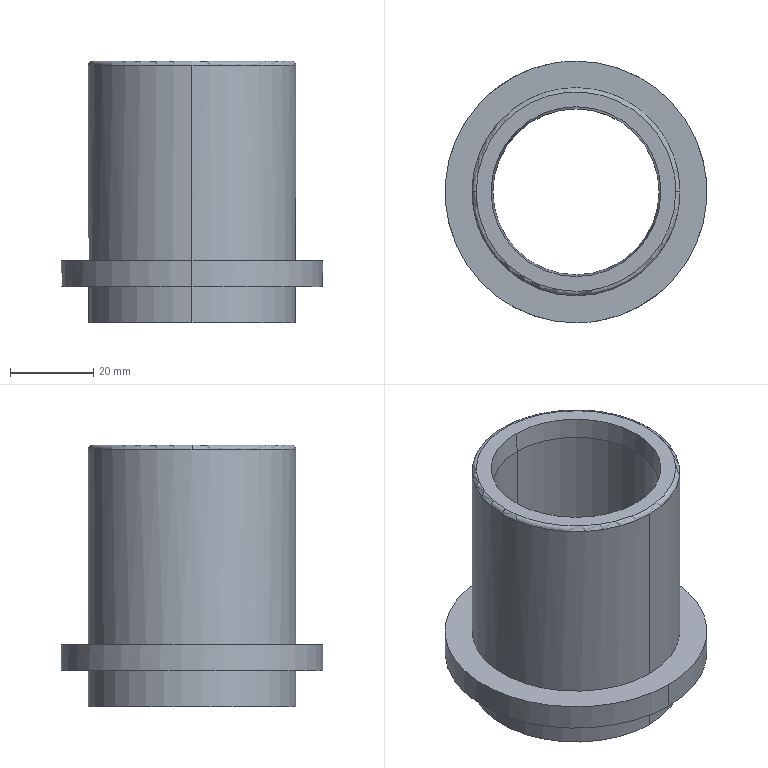Part | CATIA | 1 solid | 18 faces | box 63 x 63 x 63 mm | volume 51378 mm3 | cylinder 8 | plane 4 | torus 4 | cone 2 | commonest cylinder face diameters 50 x4 40 x2 63 x2
STEP:
#1=CARTESIAN_POINT('',(0.,-20.437,48.));
#2=VERTEX_POINT('',#1);
#3=CARTESIAN_POINT('',(0.,-20.,43.));
#4=VERTEX_POINT('',#3);
#5=CARTESIAN_POINT('',(0.,-43587.981,498027.299));
#6=DIRECTION('',(0.,-0.08716,0.9962));
#7=VECTOR('',#6,1.);
#8=LINE('',#5,#7);
#9=EDGE_CURVE('',#2,#4,#8,.F.);
#10=ORIENTED_EDGE('',*,*,#9,.F.);
#11=CARTESIAN_POINT('',(0.,20.437,48.));
#12=VERTEX_POINT('',#11);
#13=CARTESIAN_POINT('',(0.,0.,48.));
#14=DIRECTION('',(0.,0.,1.));
#15=AXIS2_PLACEMENT_3D('',#13,#14,$);
#16=CIRCLE('',#15,20.437);
#17=EDGE_CURVE('',#12,#2,#16,.F.);
#18=ORIENTED_EDGE('',*,*,#17,.F.);
#19=CARTESIAN_POINT('',(0.,20.,43.));
#20=VERTEX_POINT('',#19);
#21=CARTESIAN_POINT('',(0.,43587.981,498027.299));
#22=DIRECTION('',(0.,0.08716,0.9962));
#23=VECTOR('',#22,1.);
#24=LINE('',#21,#23);
#25=EDGE_CURVE('',#20,#12,#24,.T.);
#26=ORIENTED_EDGE('',*,*,#25,.F.);
#27=CARTESIAN_POINT('',(0.,0.,43.));
#28=DIRECTION('',(0.,0.,1.));
#29=AXIS2_PLACEMENT_3D('',#27,#28,$);
#30=CIRCLE('',#29,20.);
#31=EDGE_CURVE('',#20,#4,#30,.F.);
#32=ORIENTED_EDGE('',*,*,#31,.T.);
#33=EDGE_LOOP('',(#10,#18,#26,#32));
#34=FACE_OUTER_BOUND('',#33,.T.);
#35=CARTESIAN_POINT('',(0.,0.,45.5));
#36=DIRECTION('',(0.,0.,1.));
#37=DIRECTION('',(0.,-1.,0.));
#38=AXIS2_PLACEMENT_3D('',#35,#36,#37);
#39=CONICAL_SURFACE('',#38,20.219,0.08727);
#40=ADVANCED_FACE('',(#34),#39,.F.);
#41=ORIENTED_EDGE('',*,*,#9,.T.);
#42=CARTESIAN_POINT('',(0.,0.,43.));
#43=DIRECTION('',(0.,0.,1.));
#44=AXIS2_PLACEMENT_3D('',#42,#43,$);
#45=CIRCLE('',#44,20.);
#46=EDGE_CURVE('',#4,#20,#45,.F.);
#47=ORIENTED_EDGE('',*,*,#46,.T.);
#48=ORIENTED_EDGE('',*,*,#25,.T.);
#49=CARTESIAN_POINT('',(0.,0.,48.));
#50=DIRECTION('',(0.,0.,1.));
#51=AXIS2_PLACEMENT_3D('',#49,#50,$);
#52=CIRCLE('',#51,20.437);
#53=EDGE_CURVE('',#2,#12,#52,.F.);
#54=ORIENTED_EDGE('',*,*,#53,.F.);
#55=EDGE_LOOP('',(#41,#47,#48,#54));
#56=FACE_OUTER_BOUND('',#55,.T.);
#57=CARTESIAN_POINT('',(0.,0.,45.5));
#58=DIRECTION('',(0.,0.,1.));
#59=DIRECTION('',(0.,1.,0.));
#60=AXIS2_PLACEMENT_3D('',#57,#58,#59);
#61=CONICAL_SURFACE('',#60,20.219,0.08727);
#62=ADVANCED_FACE('',(#56),#61,.F.);
#63=CARTESIAN_POINT('',(0.,-24.,48.));
#64=VERTEX_POINT('',#63);
#65=CARTESIAN_POINT('',(-24.,-0.000000001,48.));
#66=VERTEX_POINT('',#65);
#67=CARTESIAN_POINT('',(0.,-24.,48.));
#68=CARTESIAN_POINT('',(-2.4,-24.,48.));
#69=CARTESIAN_POINT('',(-4.8,-23.7,48.));
#70=CARTESIAN_POINT('',(-7.15,-23.1,48.));
#71=CARTESIAN_POINT('',(-11.65,-21.325,48.));
#72=CARTESIAN_POINT('',(-15.575,-18.498,48.));
#73=CARTESIAN_POINT('',(-17.349,-16.844,48.));
#74=CARTESIAN_POINT('',(-20.448,-13.129,48.));
#75=CARTESIAN_POINT('',(-22.536,-8.766,48.));
#76=CARTESIAN_POINT('',(-23.301,-6.464,48.));
#77=CARTESIAN_POINT('',(-23.836,-3.756,48.));
#78=CARTESIAN_POINT('',(-23.982,-1.02,48.));
#79=CARTESIAN_POINT('',(-23.994,-0.6796,48.));
#80=CARTESIAN_POINT('',(-24.,-0.3398,48.));
#81=CARTESIAN_POINT('',(-24.,-0.000000001,48.));
#82=B_SPLINE_CURVE_WITH_KNOTS('',5,(#67,#68,#69,#70,#71,#72,#73,#74,#75,#76,#77,#78,#79,#80,#81),.UNSPECIFIED.,.F.,.U.,(6,3,3,3,6),(0.,17.012,34.025,51.037,53.446),.UNSPECIFIED.);
#83=EDGE_CURVE('',#64,#66,#82,.T.);
#84=ORIENTED_EDGE('',*,*,#83,.F.);
#85=CARTESIAN_POINT('',(24.,-0.000000001,48.));
#86=VERTEX_POINT('',#85);
#87=CARTESIAN_POINT('',(24.,-0.000000001,48.));
#88=CARTESIAN_POINT('',(24.,-2.4,48.));
#89=CARTESIAN_POINT('',(23.7,-4.8,48.));
#90=CARTESIAN_POINT('',(23.1,-7.15,48.));
#91=CARTESIAN_POINT('',(21.325,-11.65,48.));
#92=CARTESIAN_POINT('',(18.498,-15.575,48.));
#93=CARTESIAN_POINT('',(16.844,-17.349,48.));
#94=CARTESIAN_POINT('',(13.129,-20.448,48.));
#95=CARTESIAN_POINT('',(8.766,-22.536,48.));
#96=CARTESIAN_POINT('',(6.464,-23.301,48.));
#97=CARTESIAN_POINT('',(3.756,-23.836,48.));
#98=CARTESIAN_POINT('',(1.02,-23.982,48.));
#99=CARTESIAN_POINT('',(0.6796,-23.994,48.));
#100=CARTESIAN_POINT('',(0.3398,-24.,48.));
#101=CARTESIAN_POINT('',(0.,-24.,48.));
#102=B_SPLINE_CURVE_WITH_KNOTS('',5,(#87,#88,#89,#90,#91,#92,#93,#94,#95,#96,#97,#98,#99,#100,#101),.UNSPECIFIED.,.F.,.U.,(6,3,3,3,6),(0.,17.012,34.025,51.037,53.446),.UNSPECIFIED.);
#103=EDGE_CURVE('',#86,#64,#102,.T.);
#104=ORIENTED_EDGE('',*,*,#103,.F.);
#105=CARTESIAN_POINT('',(-24.,-0.000000001,48.));
#106=CARTESIAN_POINT('',(-24.,2.4,48.));
#107=CARTESIAN_POINT('',(-23.7,4.8,48.));
#108=CARTESIAN_POINT('',(-23.1,7.15,48.));
#109=CARTESIAN_POINT('',(-21.325,11.65,48.));
#110=CARTESIAN_POINT('',(-18.498,15.575,48.));
#111=CARTESIAN_POINT('',(-16.844,17.349,48.));
#112=CARTESIAN_POINT('',(-13.129,20.448,48.));
#113=CARTESIAN_POINT('',(-8.766,22.536,48.));
#114=CARTESIAN_POINT('',(-6.464,23.301,48.));
#115=CARTESIAN_POINT('',(-1.719,24.239,48.));
#116=CARTESIAN_POINT('',(3.111,23.98,48.));
#117=CARTESIAN_POINT('',(5.498,23.548,48.));
#118=CARTESIAN_POINT('',(10.112,22.096,48.));
#119=CARTESIAN_POINT('',(14.227,19.553,48.));
#120=CARTESIAN_POINT('',(16.114,18.029,48.));
#121=CARTESIAN_POINT('',(19.468,14.543,48.));
#122=CARTESIAN_POINT('',(21.86,10.339,48.));
#123=CARTESIAN_POINT('',(22.785,8.097,48.));
#124=CARTESIAN_POINT('',(23.601,5.103,48.));
#125=CARTESIAN_POINT('',(23.928,2.039,48.));
#126=CARTESIAN_POINT('',(23.976,1.359,48.));
#127=CARTESIAN_POINT('',(24.,0.6793,48.));
#128=CARTESIAN_POINT('',(24.,-0.000000001,48.));
#129=B_SPLINE_CURVE_WITH_KNOTS('',5,(#105,#106,#107,#108,#109,#110,#111,#112,#113,#114,#115,#116,#117,#118,#119,#120,#121,#122,#123,#124,#125,#126,#127,#128),.UNSPECIFIED.,.F.,.U.,(6,3,3,3,3,3,3,6),(0.,17.013,34.025,51.038,68.051,85.063,102.076,106.892),.UNSPECIFIED.);
#130=EDGE_CURVE('',#66,#86,#129,.T.);
#131=ORIENTED_EDGE('',*,*,#130,.F.);
#132=EDGE_LOOP('',(#84,#104,#131));
#133=FACE_OUTER_BOUND('',#132,.T.);
#134=ORIENTED_EDGE('',*,*,#53,.T.);
#135=ORIENTED_EDGE('',*,*,#17,.T.);
#136=EDGE_LOOP('',(#134,#135));
#137=FACE_BOUND('',#136,.T.);
#138=CARTESIAN_POINT('',(0.,-22.219,48.));
#139=DIRECTION('',(0.,0.,1.));
#140=DIRECTION('',(0.,1.,0.));
#141=AXIS2_PLACEMENT_3D('',#138,#139,#140);
#142=PLANE('',#141);
#143=ADVANCED_FACE('',(#133,#137),#142,.T.);
#144=CARTESIAN_POINT('',(0.,-20.,-12.));
#145=VERTEX_POINT('',#144);
#146=CARTESIAN_POINT('',(0.,-20.,15.5));
#147=DIRECTION('',(0.,0.,1.));
#148=VECTOR('',#147,1.);
#149=LINE('',#146,#148);
#150=EDGE_CURVE('',#4,#145,#149,.F.);
#151=ORIENTED_EDGE('',*,*,#150,.F.);
#152=ORIENTED_EDGE('',*,*,#31,.F.);
#153=CARTESIAN_POINT('',(0.,20.,-12.));
#154=VERTEX_POINT('',#153);
#155=CARTESIAN_POINT('',(0.,20.,15.5));
#156=DIRECTION('',(0.,0.,1.));
#157=VECTOR('',#156,1.);
#158=LINE('',#155,#157);
#159=EDGE_CURVE('',#154,#20,#158,.T.);
#160=ORIENTED_EDGE('',*,*,#159,.F.);
#161=CARTESIAN_POINT('',(20.,0.,-12.));
#162=VERTEX_POINT('',#161);
#163=CARTESIAN_POINT('',(0.,0.,-12.));
#164=DIRECTION('',(0.,0.,1.));
#165=AXIS2_PLACEMENT_3D('',#163,#164,$);
#166=CIRCLE('',#165,20.);
#167=EDGE_CURVE('',#154,#162,#166,.F.);
#168=ORIENTED_EDGE('',*,*,#167,.T.);
#169=CARTESIAN_POINT('',(0.,0.,-12.));
#170=DIRECTION('',(0.,0.,1.));
#171=AXIS2_PLACEMENT_3D('',#169,#170,$);
#172=CIRCLE('',#171,20.);
#173=EDGE_CURVE('',#162,#145,#172,.F.);
#174=ORIENTED_EDGE('',*,*,#173,.T.);
#175=EDGE_LOOP('',(#151,#152,#160,#168,#174));
#176=FACE_OUTER_BOUND('',#175,.T.);
#177=CARTESIAN_POINT('',(0.,0.,15.5));
#178=DIRECTION('',(0.,0.,1.));
#179=DIRECTION('',(0.,-1.,0.));
#180=AXIS2_PLACEMENT_3D('',#177,#178,#179);
#181=CYLINDRICAL_SURFACE('',#180,20.);
#182=ADVANCED_FACE('',(#176),#181,.F.);
#183=ORIENTED_EDGE('',*,*,#150,.T.);
#184=CARTESIAN_POINT('',(-20.,0.,-12.));
#185=VERTEX_POINT('',#184);
#186=CARTESIAN_POINT('',(0.,0.,-12.));
#187=DIRECTION('',(0.,0.,1.));
#188=AXIS2_PLACEMENT_3D('',#186,#187,$);
#189=CIRCLE('',#188,20.);
#190=EDGE_CURVE('',#145,#185,#189,.F.);
#191=ORIENTED_EDGE('',*,*,#190,.T.);
#192=CARTESIAN_POINT('',(0.,0.,-12.));
#193=DIRECTION('',(0.,0.,1.));
#194=AXIS2_PLACEMENT_3D('',#192,#193,$);
#195=CIRCLE('',#194,20.);
#196=EDGE_CURVE('',#185,#154,#195,.F.);
#197=ORIENTED_EDGE('',*,*,#196,.T.);
#198=ORIENTED_EDGE('',*,*,#159,.T.);
#199=ORIENTED_EDGE('',*,*,#46,.F.);
#200=EDGE_LOOP('',(#183,#191,#197,#198,#199));
#201=FACE_OUTER_BOUND('',#200,.T.);
#202=CARTESIAN_POINT('',(0.,0.,15.5));
#203=DIRECTION('',(0.,0.,1.));
#204=DIRECTION('',(0.,1.,0.));
#205=AXIS2_PLACEMENT_3D('',#202,#203,#204);
#206=CYLINDRICAL_SURFACE('',#205,20.);
#207=ADVANCED_FACE('',(#201),#206,.F.);
#208=CARTESIAN_POINT('',(-25.,0.,47.));
#209=VERTEX_POINT('',#208);
#210=CARTESIAN_POINT('',(-24.,0.,47.));
#211=DIRECTION('',(0.,-1.,0.));
#212=AXIS2_PLACEMENT_3D('',#210,#211,$);
#213=CIRCLE('',#212,1.);
#214=EDGE_CURVE('',#66,#209,#213,.T.);
#215=ORIENTED_EDGE('',*,*,#214,.T.);
#216=CARTESIAN_POINT('',(0.,-25.,47.));
#217=VERTEX_POINT('',#216);
#218=CARTESIAN_POINT('',(0.,0.,47.));
#219=DIRECTION('',(0.,0.,-1.));
#220=AXIS2_PLACEMENT_3D('',#218,#219,$);
#221=CIRCLE('',#220,25.);
#222=EDGE_CURVE('',#217,#209,#221,.T.);
#223=ORIENTED_EDGE('',*,*,#222,.F.);
#224=CARTESIAN_POINT('',(25.,0.,47.));
#225=VERTEX_POINT('',#224);
#226=CARTESIAN_POINT('',(0.,0.,47.));
#227=DIRECTION('',(0.,0.,-1.));
#228=AXIS2_PLACEMENT_3D('',#226,#227,$);
#229=CIRCLE('',#228,25.);
#230=EDGE_CURVE('',#225,#217,#229,.T.);
#231=ORIENTED_EDGE('',*,*,#230,.F.);
#232=CARTESIAN_POINT('',(24.,0.,47.));
#233=DIRECTION('',(0.,1.,0.));
#234=AXIS2_PLACEMENT_3D('',#232,#233,$);
#235=CIRCLE('',#234,1.);
#236=EDGE_CURVE('',#225,#86,#235,.F.);
#237=ORIENTED_EDGE('',*,*,#236,.T.);
#238=ORIENTED_EDGE('',*,*,#103,.T.);
#239=ORIENTED_EDGE('',*,*,#83,.T.);
#240=EDGE_LOOP('',(#215,#223,#231,#237,#238,#239));
#241=FACE_OUTER_BOUND('',#240,.T.);
#242=CARTESIAN_POINT('',(0.,0.,47.));
#243=DIRECTION('',(0.,0.,-1.));
#244=DIRECTION('',(1.,0.,0.));
#245=AXIS2_PLACEMENT_3D('',#242,#243,#244);
#246=TOROIDAL_SURFACE('',#245,24.,1.);
#247=ADVANCED_FACE('',(#241),#246,.T.);
#248=ORIENTED_EDGE('',*,*,#214,.F.);
#249=ORIENTED_EDGE('',*,*,#130,.T.);
#250=ORIENTED_EDGE('',*,*,#236,.F.);
#251=CARTESIAN_POINT('',(0.,25.,47.));
#252=VERTEX_POINT('',#251);
#253=CARTESIAN_POINT('',(0.,0.,47.));
#254=DIRECTION('',(0.,0.,-1.));
#255=AXIS2_PLACEMENT_3D('',#253,#254,$);
#256=CIRCLE('',#255,25.);
#257=EDGE_CURVE('',#252,#225,#256,.T.);
#258=ORIENTED_EDGE('',*,*,#257,.F.);
#259=CARTESIAN_POINT('',(0.,0.,47.));
#260=DIRECTION('',(0.,0.,-1.));
#261=AXIS2_PLACEMENT_3D('',#259,#260,$);
#262=CIRCLE('',#261,25.);
#263=EDGE_CURVE('',#209,#252,#262,.T.);
#264=ORIENTED_EDGE('',*,*,#263,.F.);
#265=EDGE_LOOP('',(#248,#249,#250,#258,#264));
#266=FACE_OUTER_BOUND('',#265,.T.);
#267=CARTESIAN_POINT('',(0.,0.,47.));
#268=DIRECTION('',(0.,0.,-1.));
#269=DIRECTION('',(-1.,0.,0.));
#270=AXIS2_PLACEMENT_3D('',#267,#268,#269);
#271=TOROIDAL_SURFACE('',#270,24.,1.);
#272=ADVANCED_FACE('',(#266),#271,.T.);
#273=CARTESIAN_POINT('',(-23.,0.,-15.));
#274=VERTEX_POINT('',#273);
#275=CARTESIAN_POINT('',(-23.,0.,-12.));
#276=DIRECTION('',(0.,-1.,0.));
#277=AXIS2_PLACEMENT_3D('',#275,#276,$);
#278=CIRCLE('',#277,3.);
#279=EDGE_CURVE('',#274,#185,#278,.T.);
#280=ORIENTED_EDGE('',*,*,#279,.F.);
#281=CARTESIAN_POINT('',(23.,0.,-15.));
#282=VERTEX_POINT('',#281);
#283=CARTESIAN_POINT('',(0.,0.,-15.));
#284=DIRECTION('',(0.,0.,-1.));
#285=AXIS2_PLACEMENT_3D('',#283,#284,$);
#286=CIRCLE('',#285,23.);
#287=EDGE_CURVE('',#274,#282,#286,.T.);
#288=ORIENTED_EDGE('',*,*,#287,.T.);
#289=CARTESIAN_POINT('',(23.,0.,-12.));
#290=DIRECTION('',(0.,1.,0.));
#291=AXIS2_PLACEMENT_3D('',#289,#290,$);
#292=CIRCLE('',#291,3.);
#293=EDGE_CURVE('',#162,#282,#292,.F.);
#294=ORIENTED_EDGE('',*,*,#293,.F.);
#295=ORIENTED_EDGE('',*,*,#167,.F.);
#296=ORIENTED_EDGE('',*,*,#196,.F.);
#297=EDGE_LOOP('',(#280,#288,#294,#295,#296));
#298=FACE_OUTER_BOUND('',#297,.T.);
#299=CARTESIAN_POINT('',(0.,0.,-12.));
#300=DIRECTION('',(0.,0.,-1.));
#301=DIRECTION('',(-1.,0.,0.));
#302=AXIS2_PLACEMENT_3D('',#299,#300,#301);
#303=TOROIDAL_SURFACE('',#302,23.,3.);
#304=ADVANCED_FACE('',(#298),#303,.T.);
#305=ORIENTED_EDGE('',*,*,#279,.T.);
#306=ORIENTED_EDGE('',*,*,#190,.F.);
#307=ORIENTED_EDGE('',*,*,#173,.F.);
#308=ORIENTED_EDGE('',*,*,#293,.T.);
#309=CARTESIAN_POINT('',(0.,-23.,-15.));
#310=VERTEX_POINT('',#309);
#311=CARTESIAN_POINT('',(0.,0.,-15.));
#312=DIRECTION('',(0.,0.,-1.));
#313=AXIS2_PLACEMENT_3D('',#311,#312,$);
#314=CIRCLE('',#313,23.);
#315=EDGE_CURVE('',#282,#310,#314,.T.);
#316=ORIENTED_EDGE('',*,*,#315,.T.);
#317=CARTESIAN_POINT('',(0.,0.,-15.));
#318=DIRECTION('',(0.,0.,-1.));
#319=AXIS2_PLACEMENT_3D('',#317,#318,$);
#320=CIRCLE('',#319,23.);
#321=EDGE_CURVE('',#310,#274,#320,.T.);
#322=ORIENTED_EDGE('',*,*,#321,.T.);
#323=EDGE_LOOP('',(#305,#306,#307,#308,#316,#322));
#324=FACE_OUTER_BOUND('',#323,.T.);
#325=CARTESIAN_POINT('',(0.,0.,-12.));
#326=DIRECTION('',(0.,0.,-1.));
#327=DIRECTION('',(1.,0.,0.));
#328=AXIS2_PLACEMENT_3D('',#325,#326,#327);
#329=TOROIDAL_SURFACE('',#328,23.,3.);
#330=ADVANCED_FACE('',(#324),#329,.T.);
#331=CARTESIAN_POINT('',(0.,-25.,0.));
#332=VERTEX_POINT('',#331);
#333=CARTESIAN_POINT('',(0.,-25.,23.5));
#334=DIRECTION('',(0.,0.,1.));
#335=VECTOR('',#334,1.);
#336=LINE('',#333,#335);
#337=EDGE_CURVE('',#217,#332,#336,.F.);
#338=ORIENTED_EDGE('',*,*,#337,.F.);
#339=ORIENTED_EDGE('',*,*,#222,.T.);
#340=ORIENTED_EDGE('',*,*,#263,.T.);
#341=CARTESIAN_POINT('',(0.,25.,0.));
#342=VERTEX_POINT('',#341);
#343=CARTESIAN_POINT('',(0.,25.,23.5));
#344=DIRECTION('',(0.,0.,1.));
#345=VECTOR('',#344,1.);
#346=LINE('',#343,#345);
#347=EDGE_CURVE('',#342,#252,#346,.T.);
#348=ORIENTED_EDGE('',*,*,#347,.F.);
#349=CARTESIAN_POINT('',(0.,0.,0.));
#350=DIRECTION('',(0.,0.,1.));
#351=AXIS2_PLACEMENT_3D('',#349,#350,$);
#352=CIRCLE('',#351,25.);
#353=EDGE_CURVE('',#332,#342,#352,.F.);
#354=ORIENTED_EDGE('',*,*,#353,.F.);
#355=EDGE_LOOP('',(#338,#339,#340,#348,#354));
#356=FACE_OUTER_BOUND('',#355,.T.);
#357=CARTESIAN_POINT('',(0.,0.,23.5));
#358=DIRECTION('',(0.,0.,1.));
#359=DIRECTION('',(0.,1.,0.));
#360=AXIS2_PLACEMENT_3D('',#357,#358,#359);
#361=CYLINDRICAL_SURFACE('',#360,25.);
#362=ADVANCED_FACE('',(#356),#361,.T.);
#363=ORIENTED_EDGE('',*,*,#337,.T.);
#364=CARTESIAN_POINT('',(0.,0.,0.));
#365=DIRECTION('',(0.,0.,1.));
#366=AXIS2_PLACEMENT_3D('',#364,#365,$);
#367=CIRCLE('',#366,25.);
#368=EDGE_CURVE('',#342,#332,#367,.F.);
#369=ORIENTED_EDGE('',*,*,#368,.F.);
#370=ORIENTED_EDGE('',*,*,#347,.T.);
#371=ORIENTED_EDGE('',*,*,#257,.T.);
#372=ORIENTED_EDGE('',*,*,#230,.T.);
#373=EDGE_LOOP('',(#363,#369,#370,#371,#372));
#374=FACE_OUTER_BOUND('',#373,.T.);
#375=CARTESIAN_POINT('',(0.,0.,23.5));
#376=DIRECTION('',(0.,0.,1.));
#377=DIRECTION('',(0.,-1.,0.));
#378=AXIS2_PLACEMENT_3D('',#375,#376,#377);
#379=CYLINDRICAL_SURFACE('',#378,25.);
#380=ADVANCED_FACE('',(#374),#379,.T.);
#381=CARTESIAN_POINT('',(0.,-25.,-15.));
#382=VERTEX_POINT('',#381);
#383=CARTESIAN_POINT('',(0.,25.,-15.));
#384=VERTEX_POINT('',#383);
#385=CARTESIAN_POINT('',(0.,0.,-15.));
#386=DIRECTION('',(0.,0.,-1.));
#387=AXIS2_PLACEMENT_3D('',#385,#386,$);
#388=CIRCLE('',#387,25.);
#389=EDGE_CURVE('',#382,#384,#388,.T.);
#390=ORIENTED_EDGE('',*,*,#389,.T.);
#391=CARTESIAN_POINT('',(0.,0.,-15.));
#392=DIRECTION('',(0.,0.,-1.));
#393=AXIS2_PLACEMENT_3D('',#391,#392,$);
#394=CIRCLE('',#393,25.);
#395=EDGE_CURVE('',#384,#382,#394,.T.);
#396=ORIENTED_EDGE('',*,*,#395,.T.);
#397=EDGE_LOOP('',(#390,#396));
#398=FACE_OUTER_BOUND('',#397,.T.);
#399=ORIENTED_EDGE('',*,*,#321,.F.);
#400=ORIENTED_EDGE('',*,*,#315,.F.);
#401=ORIENTED_EDGE('',*,*,#287,.F.);
#402=EDGE_LOOP('',(#399,#400,#401));
#403=FACE_BOUND('',#402,.T.);
#404=CARTESIAN_POINT('',(0.,-24.,-15.));
#405=DIRECTION('',(0.,0.,-1.));
#406=DIRECTION('',(0.,-1.,0.));
#407=AXIS2_PLACEMENT_3D('',#404,#405,#406);
#408=PLANE('',#407);
#409=ADVANCED_FACE('',(#398,#403),#408,.T.);
#410=CARTESIAN_POINT('',(0.,-31.5,0.));
#411=VERTEX_POINT('',#410);
#412=CARTESIAN_POINT('',(0.,31.5,0.));
#413=VERTEX_POINT('',#412);
#414=CARTESIAN_POINT('',(0.,-31.5,0.));
#415=CARTESIAN_POINT('',(-3.024,-31.5,0.));
#416=CARTESIAN_POINT('',(-6.049,-31.137,0.));
#417=CARTESIAN_POINT('',(-9.016,-30.411,0.));
#418=CARTESIAN_POINT('',(-14.716,-28.261,0.));
#419=CARTESIAN_POINT('',(-19.746,-24.824,0.));
#420=CARTESIAN_POINT('',(-22.042,-22.809,0.));
#421=CARTESIAN_POINT('',(-26.105,-18.27,0.));
#422=CARTESIAN_POINT('',(-28.978,-12.898,0.));
#423=CARTESIAN_POINT('',(-30.084,-10.051,0.));
#424=CARTESIAN_POINT('',(-31.592,-4.148,0.));
#425=CARTESIAN_POINT('',(-31.66,1.943,0.));
#426=CARTESIAN_POINT('',(-31.326,4.98,0.));
#427=CARTESIAN_POINT('',(-29.937,10.911,0.));
#428=CARTESIAN_POINT('',(-27.183,16.346,0.));
#429=CARTESIAN_POINT('',(-25.485,18.884,0.));
#430=CARTESIAN_POINT('',(-21.513,23.504,0.));
#431=CARTESIAN_POINT('',(-16.561,27.052,0.));
#432=CARTESIAN_POINT('',(-13.882,28.52,0.));
#433=CARTESIAN_POINT('',(-9.516,30.267,0.));
#434=CARTESIAN_POINT('',(-4.926,31.178,0.));
#435=CARTESIAN_POINT('',(-3.29,31.393,0.));
#436=CARTESIAN_POINT('',(-1.645,31.5,0.));
#437=CARTESIAN_POINT('',(0.,31.5,0.));
#438=B_SPLINE_CURVE_WITH_KNOTS('',5,(#414,#415,#416,#417,#418,#419,#420,#421,#422,#423,#424,#425,#426,#427,#428,#429,#430,#431,#432,#433,#434,#435,#436,#437),.UNSPECIFIED.,.F.,.U.,(6,3,3,3,3,3,3,6),(0.,21.434,42.869,64.303,85.737,107.172,128.606,140.265),.UNSPECIFIED.);
#439=EDGE_CURVE('',#411,#413,#438,.T.);
#440=ORIENTED_EDGE('',*,*,#439,.F.);
#441=CARTESIAN_POINT('',(0.,31.5,0.));
#442=CARTESIAN_POINT('',(3.024,31.5,0.));
#443=CARTESIAN_POINT('',(6.049,31.137,0.));
#444=CARTESIAN_POINT('',(9.016,30.411,0.));
#445=CARTESIAN_POINT('',(14.716,28.261,0.));
#446=CARTESIAN_POINT('',(19.746,24.824,0.));
#447=CARTESIAN_POINT('',(22.042,22.809,0.));
#448=CARTESIAN_POINT('',(26.105,18.27,0.));
#449=CARTESIAN_POINT('',(28.978,12.898,0.));
#450=CARTESIAN_POINT('',(30.084,10.051,0.));
#451=CARTESIAN_POINT('',(31.592,4.148,0.));
#452=CARTESIAN_POINT('',(31.66,-1.943,0.));
#453=CARTESIAN_POINT('',(31.326,-4.98,0.));
#454=CARTESIAN_POINT('',(29.937,-10.911,0.));
#455=CARTESIAN_POINT('',(27.183,-16.346,0.));
#456=CARTESIAN_POINT('',(25.485,-18.884,0.));
#457=CARTESIAN_POINT('',(21.513,-23.504,0.));
#458=CARTESIAN_POINT('',(16.561,-27.052,0.));
#459=CARTESIAN_POINT('',(13.882,-28.52,0.));
#460=CARTESIAN_POINT('',(9.516,-30.267,0.));
#461=CARTESIAN_POINT('',(4.926,-31.178,0.));
#462=CARTESIAN_POINT('',(3.29,-31.393,0.));
#463=CARTESIAN_POINT('',(1.645,-31.5,0.));
#464=CARTESIAN_POINT('',(0.,-31.5,0.));
#465=B_SPLINE_CURVE_WITH_KNOTS('',5,(#441,#442,#443,#444,#445,#446,#447,#448,#449,#450,#451,#452,#453,#454,#455,#456,#457,#458,#459,#460,#461,#462,#463,#464),.UNSPECIFIED.,.F.,.U.,(6,3,3,3,3,3,3,6),(0.,21.434,42.869,64.303,85.737,107.172,128.606,140.265),.UNSPECIFIED.);
#466=EDGE_CURVE('',#413,#411,#465,.T.);
#467=ORIENTED_EDGE('',*,*,#466,.F.);
#468=EDGE_LOOP('',(#440,#467));
#469=FACE_OUTER_BOUND('',#468,.T.);
#470=ORIENTED_EDGE('',*,*,#353,.T.);
#471=ORIENTED_EDGE('',*,*,#368,.T.);
#472=EDGE_LOOP('',(#470,#471));
#473=FACE_BOUND('',#472,.T.);
#474=CARTESIAN_POINT('',(0.,-28.25,0.));
#475=DIRECTION('',(0.,0.,1.));
#476=DIRECTION('',(0.,1.,0.));
#477=AXIS2_PLACEMENT_3D('',#474,#475,#476);
#478=PLANE('',#477);
#479=ADVANCED_FACE('',(#469,#473),#478,.T.);
#480=CARTESIAN_POINT('',(0.,-25.,-6.3));
#481=VERTEX_POINT('',#480);
#482=CARTESIAN_POINT('',(0.,-25.,-10.65));
#483=DIRECTION('',(0.,0.,1.));
#484=VECTOR('',#483,1.);
#485=LINE('',#482,#484);
#486=EDGE_CURVE('',#481,#382,#485,.F.);
#487=ORIENTED_EDGE('',*,*,#486,.F.);
#488=CARTESIAN_POINT('',(0.,25.,-6.3));
#489=VERTEX_POINT('',#488);
#490=CARTESIAN_POINT('',(0.,0.,-6.3));
#491=DIRECTION('',(0.,0.,1.));
#492=AXIS2_PLACEMENT_3D('',#490,#491,$);
#493=CIRCLE('',#492,25.);
#494=EDGE_CURVE('',#481,#489,#493,.F.);
#495=ORIENTED_EDGE('',*,*,#494,.T.);
#496=CARTESIAN_POINT('',(0.,25.,-10.65));
#497=DIRECTION('',(0.,0.,1.));
#498=VECTOR('',#497,1.);
#499=LINE('',#496,#498);
#500=EDGE_CURVE('',#384,#489,#499,.T.);
#501=ORIENTED_EDGE('',*,*,#500,.F.);
#502=ORIENTED_EDGE('',*,*,#389,.F.);
#503=EDGE_LOOP('',(#487,#495,#501,#502));
#504=FACE_OUTER_BOUND('',#503,.T.);
#505=CARTESIAN_POINT('',(0.,0.,-10.65));
#506=DIRECTION('',(0.,0.,1.));
#507=DIRECTION('',(0.,1.,0.));
#508=AXIS2_PLACEMENT_3D('',#505,#506,#507);
#509=CYLINDRICAL_SURFACE('',#508,25.);
#510=ADVANCED_FACE('',(#504),#509,.T.);
#511=ORIENTED_EDGE('',*,*,#486,.T.);
#512=ORIENTED_EDGE('',*,*,#395,.F.);
#513=ORIENTED_EDGE('',*,*,#500,.T.);
#514=CARTESIAN_POINT('',(0.,0.,-6.3));
#515=DIRECTION('',(0.,0.,1.));
#516=AXIS2_PLACEMENT_3D('',#514,#515,$);
#517=CIRCLE('',#516,25.);
#518=EDGE_CURVE('',#489,#481,#517,.F.);
#519=ORIENTED_EDGE('',*,*,#518,.T.);
#520=EDGE_LOOP('',(#511,#512,#513,#519));
#521=FACE_OUTER_BOUND('',#520,.T.);
#522=CARTESIAN_POINT('',(0.,0.,-10.65));
#523=DIRECTION('',(0.,0.,1.));
#524=DIRECTION('',(0.,-1.,0.));
#525=AXIS2_PLACEMENT_3D('',#522,#523,#524);
#526=CYLINDRICAL_SURFACE('',#525,25.);
#527=ADVANCED_FACE('',(#521),#526,.T.);
#528=CARTESIAN_POINT('',(0.,-31.5,-6.3));
#529=VERTEX_POINT('',#528);
#530=CARTESIAN_POINT('',(0.,-31.5,-3.15));
#531=DIRECTION('',(0.,0.,1.));
#532=VECTOR('',#531,1.);
#533=LINE('',#530,#532);
#534=EDGE_CURVE('',#411,#529,#533,.F.);
#535=ORIENTED_EDGE('',*,*,#534,.F.);
#536=ORIENTED_EDGE('',*,*,#439,.T.);
#537=CARTESIAN_POINT('',(0.,31.5,-6.3));
#538=VERTEX_POINT('',#537);
#539=CARTESIAN_POINT('',(0.,31.5,-3.15));
#540=DIRECTION('',(0.,0.,1.));
#541=VECTOR('',#540,1.);
#542=LINE('',#539,#541);
#543=EDGE_CURVE('',#538,#413,#542,.T.);
#544=ORIENTED_EDGE('',*,*,#543,.F.);
#545=CARTESIAN_POINT('',(0.,0.,-6.3));
#546=DIRECTION('',(0.,0.,1.));
#547=AXIS2_PLACEMENT_3D('',#545,#546,$);
#548=CIRCLE('',#547,31.5);
#549=EDGE_CURVE('',#529,#538,#548,.F.);
#550=ORIENTED_EDGE('',*,*,#549,.F.);
#551=EDGE_LOOP('',(#535,#536,#544,#550));
#552=FACE_OUTER_BOUND('',#551,.T.);
#553=CARTESIAN_POINT('',(0.,0.,-3.15));
#554=DIRECTION('',(0.,0.,1.));
#555=DIRECTION('',(0.,1.,0.));
#556=AXIS2_PLACEMENT_3D('',#553,#554,#555);
#557=CYLINDRICAL_SURFACE('',#556,31.5);
#558=ADVANCED_FACE('',(#552),#557,.T.);
#559=ORIENTED_EDGE('',*,*,#534,.T.);
#560=CARTESIAN_POINT('',(0.,0.,-6.3));
#561=DIRECTION('',(0.,0.,1.));
#562=AXIS2_PLACEMENT_3D('',#560,#561,$);
#563=CIRCLE('',#562,31.5);
#564=EDGE_CURVE('',#538,#529,#563,.F.);
#565=ORIENTED_EDGE('',*,*,#564,.F.);
#566=ORIENTED_EDGE('',*,*,#543,.T.);
#567=ORIENTED_EDGE('',*,*,#466,.T.);
#568=EDGE_LOOP('',(#559,#565,#566,#567));
#569=FACE_OUTER_BOUND('',#568,.T.);
#570=CARTESIAN_POINT('',(0.,0.,-3.15));
#571=DIRECTION('',(0.,0.,1.));
#572=DIRECTION('',(0.,-1.,0.));
#573=AXIS2_PLACEMENT_3D('',#570,#571,#572);
#574=CYLINDRICAL_SURFACE('',#573,31.5);
#575=ADVANCED_FACE('',(#569),#574,.T.);
#576=ORIENTED_EDGE('',*,*,#549,.T.);
#577=ORIENTED_EDGE('',*,*,#564,.T.);
#578=EDGE_LOOP('',(#576,#577));
#579=FACE_OUTER_BOUND('',#578,.T.);
#580=ORIENTED_EDGE('',*,*,#494,.F.);
#581=ORIENTED_EDGE('',*,*,#518,.F.);
#582=EDGE_LOOP('',(#580,#581));
#583=FACE_BOUND('',#582,.T.);
#584=CARTESIAN_POINT('',(0.,-28.25,-6.3));
#585=DIRECTION('',(0.,0.,-1.));
#586=DIRECTION('',(0.,-1.,0.));
#587=AXIS2_PLACEMENT_3D('',#584,#585,#586);
#588=PLANE('',#587);
#589=ADVANCED_FACE('',(#579,#583),#588,.T.);
#590=CLOSED_SHELL('',(#40,#62,#143,#182,#207,#247,#272,#304,#330,#362,#380,#409,#479,#510,#527,#558,#575,#589));
#591=MANIFOLD_SOLID_BREP('',#590);
#592=(LENGTH_UNIT()NAMED_UNIT(*)SI_UNIT(.MILLI.,.METRE.));
#593=UNCERTAINTY_MEASURE_WITH_UNIT(LENGTH_MEASURE(0.005),#592,'','');
#594=(NAMED_UNIT(*)PLANE_ANGLE_UNIT()SI_UNIT($,.RADIAN.));
#595=(NAMED_UNIT(*)SI_UNIT($,.STERADIAN.)SOLID_ANGLE_UNIT());
#596=(GEOMETRIC_REPRESENTATION_CONTEXT(3)GLOBAL_UNCERTAINTY_ASSIGNED_CONTEXT((#593))GLOBAL_UNIT_ASSIGNED_CONTEXT((#592,#594,#595))REPRESENTATION_CONTEXT('',''));
#597=ADVANCED_BREP_SHAPE_REPRESENTATION('',(#591),#596);